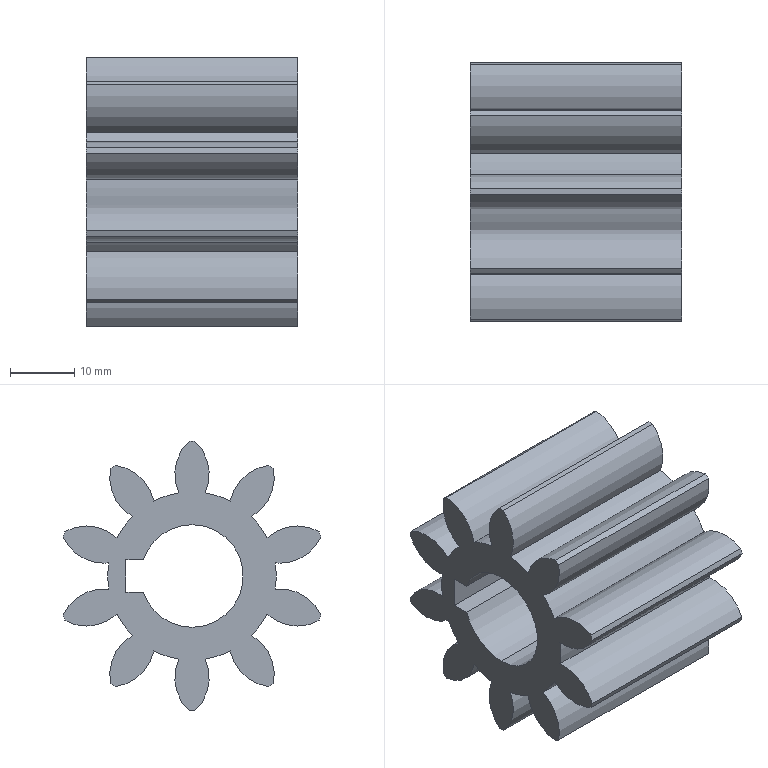Part | SolidWorks | features Extrusion 1 | 1 solid | 53 faces | box 33 x 40.213 x 42 mm | volume 22176 mm3 | cylinder 48 | plane 5 | commonest cylinder face diameters 14 x24 42 x11 26.248 x10 16 x3